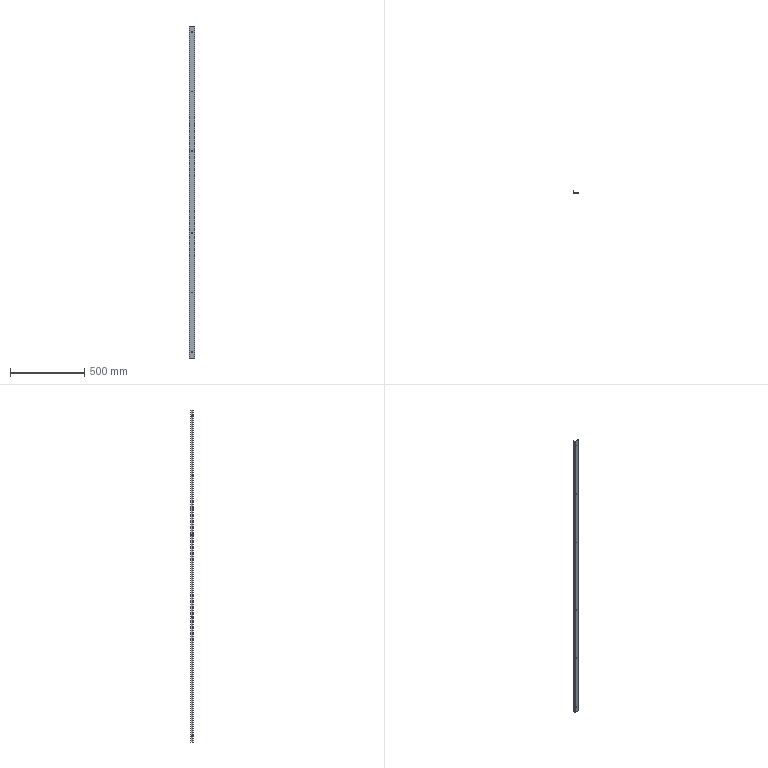Part | SolidWorks | features ICE 2, FlatPattern 1, SMBaseFlange 1, SheetMetal 1 | 1 solid | 56 faces | box 39 x 15 x 2234 mm | volume 228036 mm3 | cylinder 32 | plane 24 | commonest cylinder face diameters 4.5 x18 4.2 x12 2 x1 6 x1